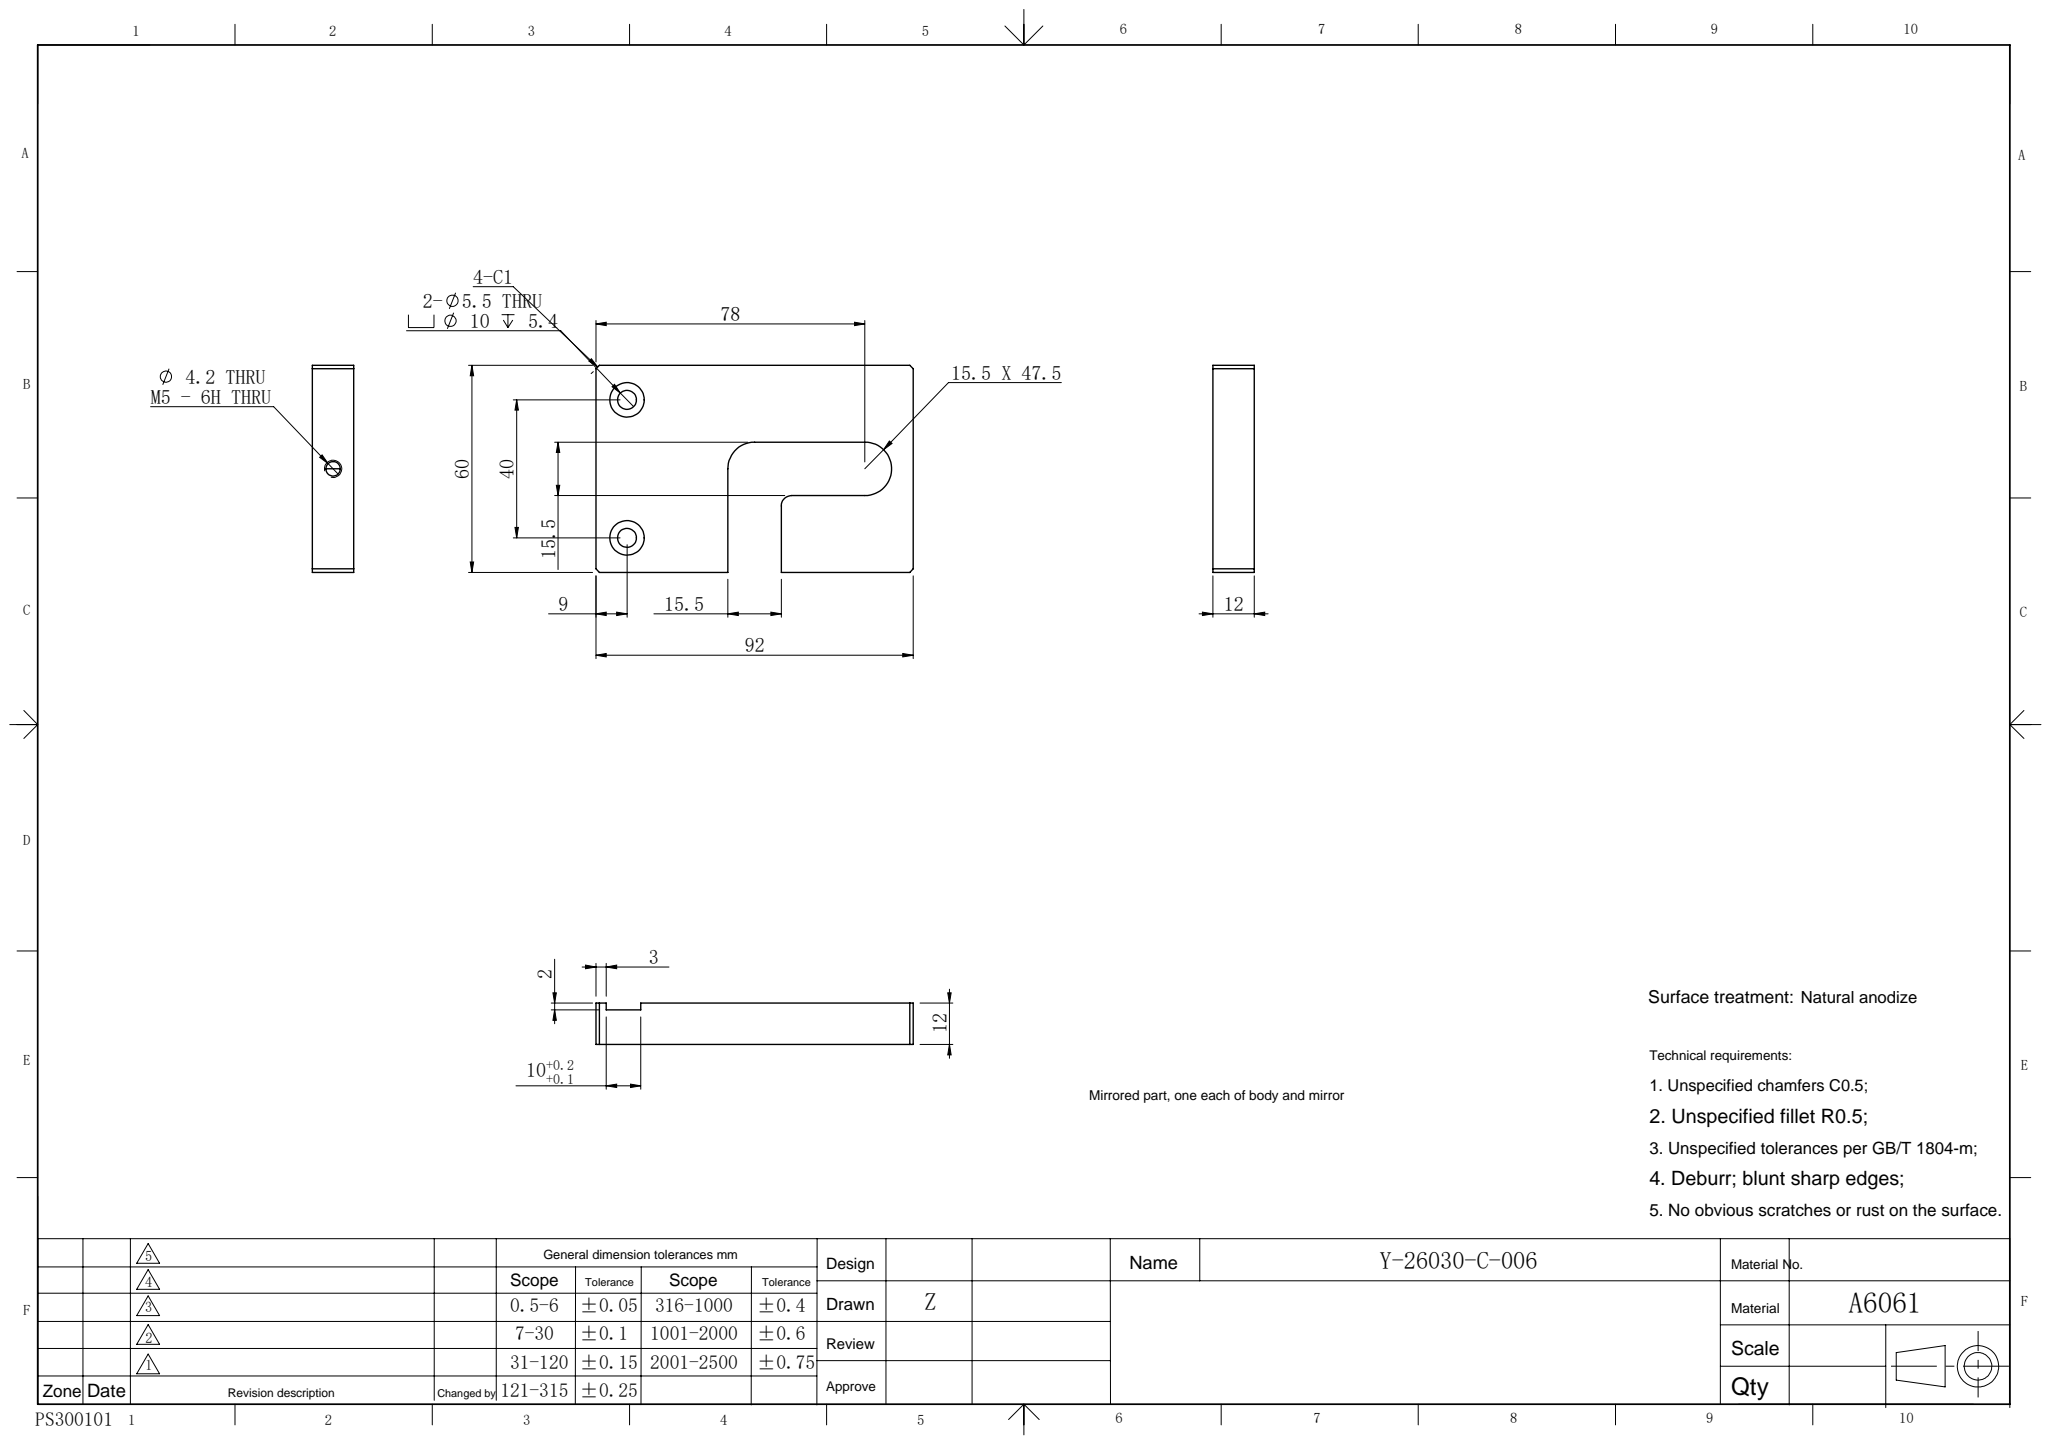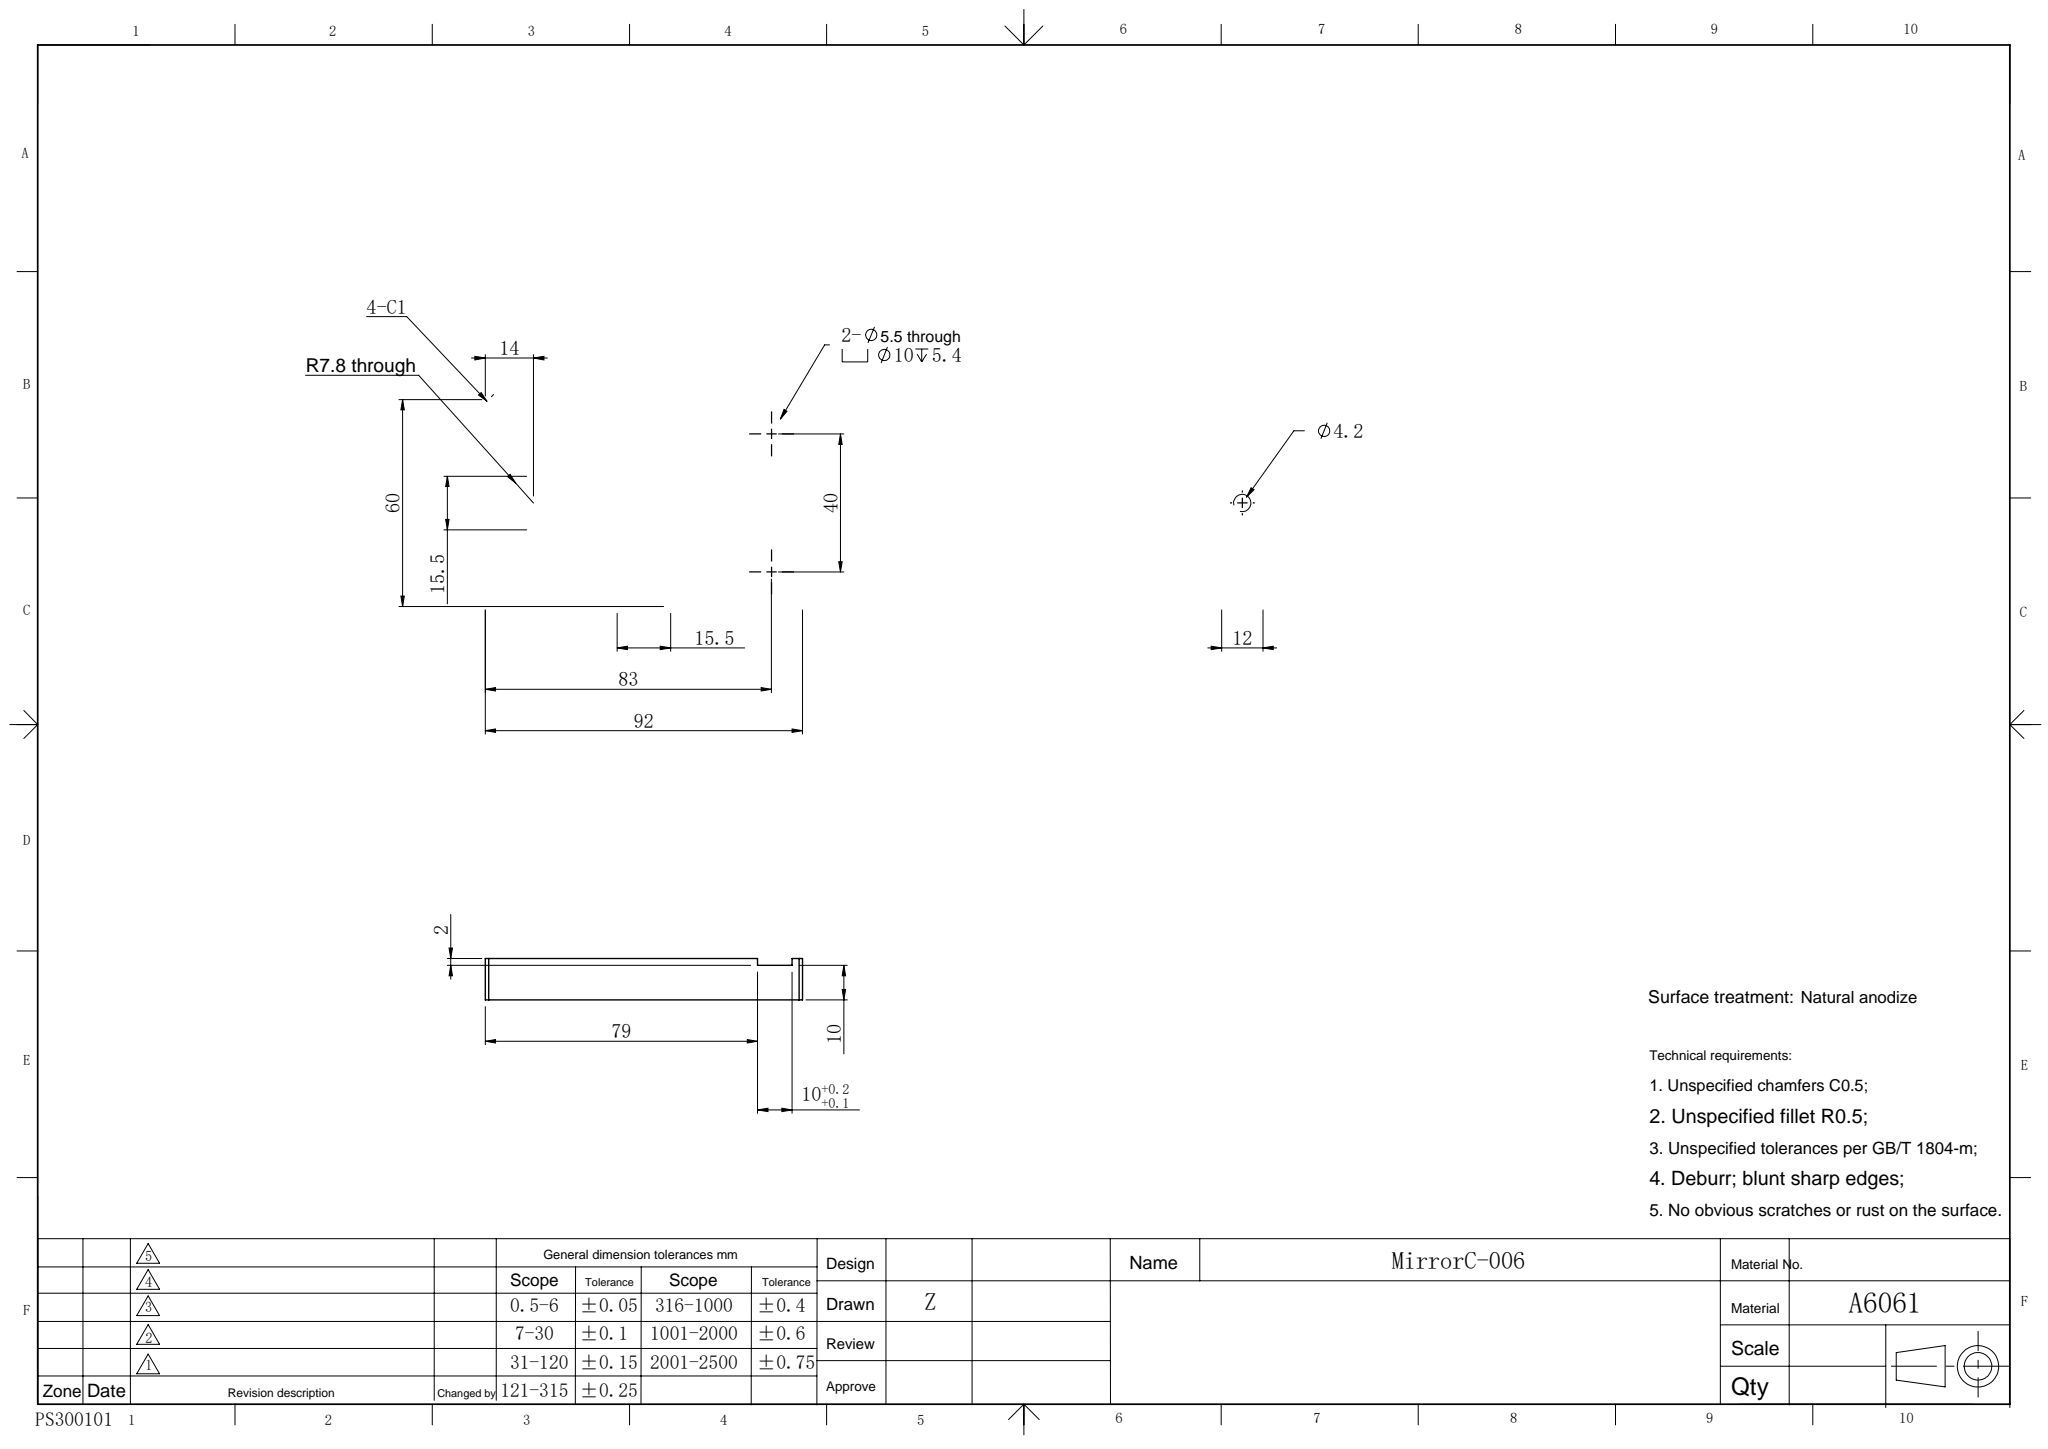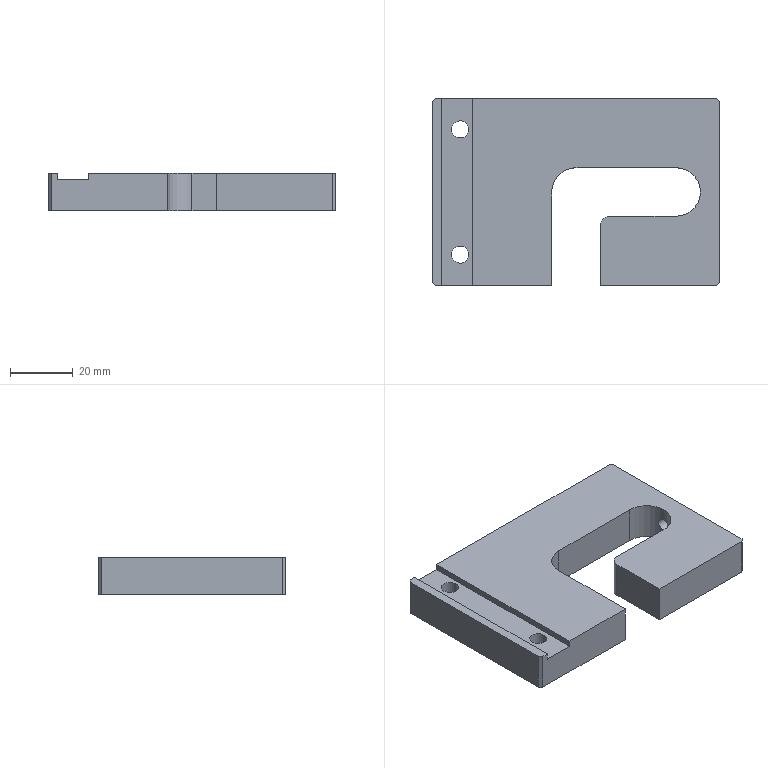Part | SolidWorks | features MirrorStock 1 | 1 solid | 35 faces | box 92 x 60 x 12 mm | volume 51329 mm3 | plane 21 | cylinder 14 | commonest cylinder face diameters 5.5 x4 10 x4 15.5 x3 4.2 x2 6 x1